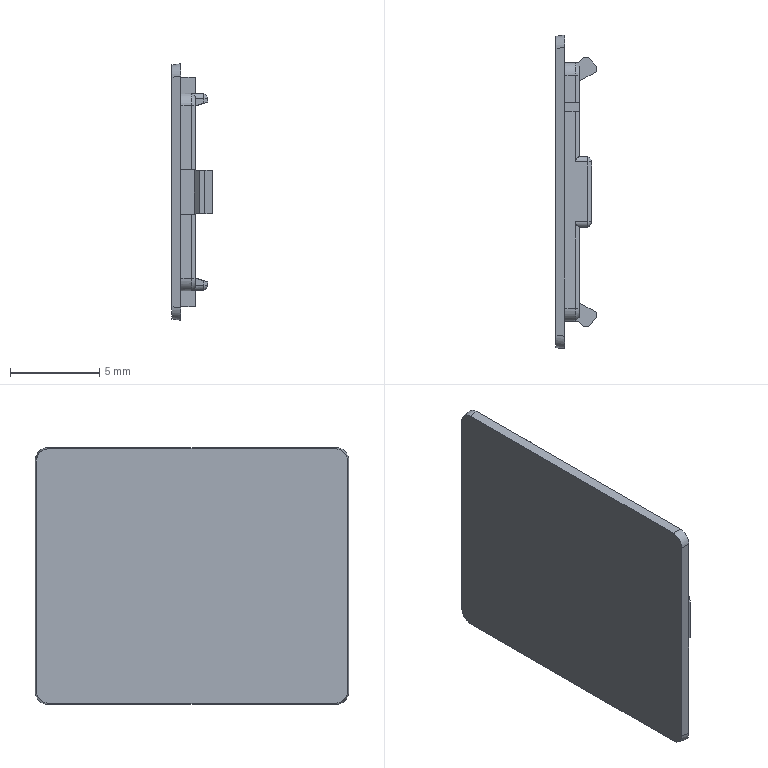Part | STEP file | [LR-XN11P]-Part-2 | 1 solid | 116 faces | box 2.25 x 17.6 x 14.4 mm | volume 152.141 mm3 | plane 92 | cylinder 16 | spline 8 | commonest cylinder face diameters 1.4 x8 0.4 x4 0.6 x4